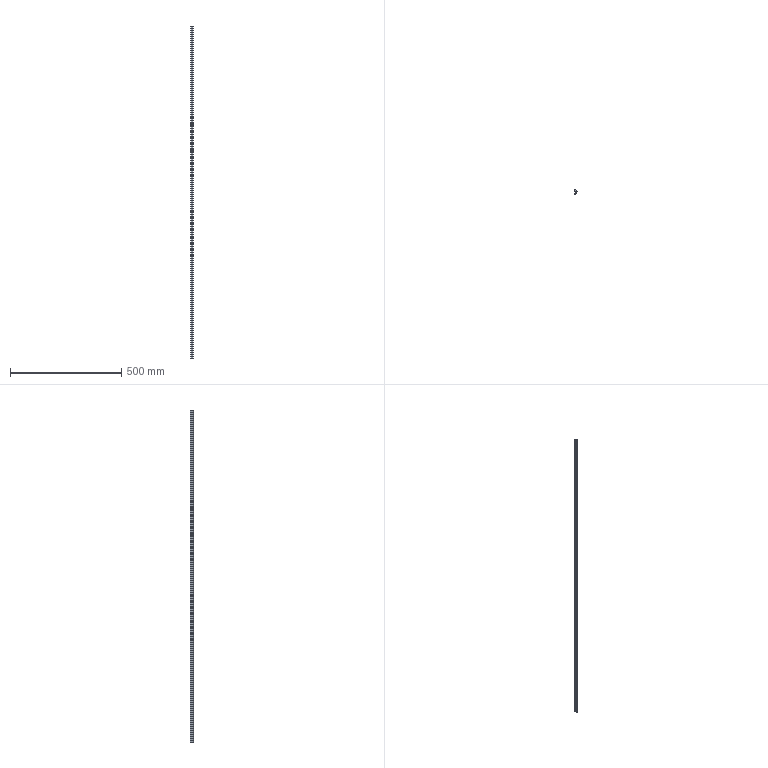Part | SolidWorks | features BaseBody 1, MoveFace 1 | 1 solid | 20 faces | box 10.8 x 17.5 x 1495 mm | volume 117807 mm3 | cylinder 11 | plane 9 | commonest cylinder face diameters 1.6 x2 14 x2 0.4 x1 0.6 x1 0.8 x1 2.6 x1
STEP:
#1=CARTESIAN_POINT('',(-3.236,-11.055,1395.));
#2=VERTEX_POINT('',#1);
#3=CARTESIAN_POINT('',(-4.3,-10.3,1395.));
#4=VERTEX_POINT('',#3);
#5=CARTESIAN_POINT('',(-3.5,-10.3,1395.));
#6=DIRECTION('',(0.,0.,-1.));
#7=DIRECTION('',(1.,0.,0.));
#8=AXIS2_PLACEMENT_3D('',#5,#6,#7);
#9=CIRCLE('',#8,0.8);
#10=EDGE_CURVE('',#2,#4,#9,.T.);
#11=ORIENTED_EDGE('',*,*,#10,.T.);
#12=CARTESIAN_POINT('',(-4.3,-10.3,-100.));
#13=VERTEX_POINT('',#12);
#14=CARTESIAN_POINT('',(-4.3,-10.3,-100.));
#15=DIRECTION('',(0.,0.,-1.));
#16=VECTOR('',#15,1000.);
#17=LINE('',#14,#16);
#18=EDGE_CURVE('',#4,#13,#17,.T.);
#19=ORIENTED_EDGE('',*,*,#18,.T.);
#20=CARTESIAN_POINT('',(-3.236,-11.055,-100.));
#21=VERTEX_POINT('',#20);
#22=CARTESIAN_POINT('',(-3.5,-10.3,-100.));
#23=DIRECTION('',(0.,0.,1.));
#24=DIRECTION('',(-1.,0.,0.));
#25=AXIS2_PLACEMENT_3D('',#22,#23,#24);
#26=CIRCLE('',#25,0.8);
#27=EDGE_CURVE('',#13,#21,#26,.T.);
#28=ORIENTED_EDGE('',*,*,#27,.T.);
#29=CARTESIAN_POINT('',(-3.236,-11.055,-100.));
#30=DIRECTION('',(0.,0.,-1.));
#31=VECTOR('',#30,1000.);
#32=LINE('',#29,#31);
#33=EDGE_CURVE('',#2,#21,#32,.T.);
#34=ORIENTED_EDGE('',*,*,#33,.F.);
#35=EDGE_LOOP('',(#11,#19,#28,#34));
#36=FACE_OUTER_BOUND('',#35,.T.);
#37=CARTESIAN_POINT('',(-3.5,-10.3,-100.));
#38=DIRECTION('',(0.,0.,-1.));
#39=DIRECTION('',(-1.,0.,0.));
#40=AXIS2_PLACEMENT_3D('',#37,#38,#39);
#41=CYLINDRICAL_SURFACE('',#40,0.8);
#42=ADVANCED_FACE('',(#36),#41,.T.);
#43=CARTESIAN_POINT('',(1.184,-6.397,-100.));
#44=VERTEX_POINT('',#43);
#45=CARTESIAN_POINT('',(-5.702,-4.29,-100.));
#46=DIRECTION('',(0.,0.,1.));
#47=DIRECTION('',(-1.,0.,0.));
#48=AXIS2_PLACEMENT_3D('',#45,#46,#47);
#49=CIRCLE('',#48,7.201);
#50=EDGE_CURVE('',#21,#44,#49,.T.);
#51=ORIENTED_EDGE('',*,*,#50,.T.);
#52=CARTESIAN_POINT('',(1.184,-6.397,1395.));
#53=VERTEX_POINT('',#52);
#54=CARTESIAN_POINT('',(1.184,-6.397,-100.));
#55=DIRECTION('',(0.,0.,1.));
#56=VECTOR('',#55,1000.);
#57=LINE('',#54,#56);
#58=EDGE_CURVE('',#44,#53,#57,.T.);
#59=ORIENTED_EDGE('',*,*,#58,.T.);
#60=CARTESIAN_POINT('',(-5.702,-4.29,1395.));
#61=DIRECTION('',(0.,0.,-1.));
#62=DIRECTION('',(1.,0.,0.));
#63=AXIS2_PLACEMENT_3D('',#60,#61,#62);
#64=CIRCLE('',#63,7.201);
#65=EDGE_CURVE('',#53,#2,#64,.T.);
#66=ORIENTED_EDGE('',*,*,#65,.T.);
#67=ORIENTED_EDGE('',*,*,#33,.T.);
#68=EDGE_LOOP('',(#51,#59,#66,#67));
#69=FACE_OUTER_BOUND('',#68,.T.);
#70=CARTESIAN_POINT('',(-5.702,-4.29,-100.));
#71=DIRECTION('',(0.,0.,-1.));
#72=DIRECTION('',(-1.,0.,0.));
#73=AXIS2_PLACEMENT_3D('',#70,#71,#72);
#74=CYLINDRICAL_SURFACE('',#73,7.201);
#75=ADVANCED_FACE('',(#69),#74,.T.);
#76=CARTESIAN_POINT('',(0.9,-6.,-100.));
#77=VERTEX_POINT('',#76);
#78=CARTESIAN_POINT('',(0.9,-6.3,-100.));
#79=DIRECTION('',(0.,0.,1.));
#80=DIRECTION('',(-1.,0.,0.));
#81=AXIS2_PLACEMENT_3D('',#78,#79,#80);
#82=CIRCLE('',#81,0.3);
#83=EDGE_CURVE('',#44,#77,#82,.T.);
#84=ORIENTED_EDGE('',*,*,#83,.T.);
#85=CARTESIAN_POINT('',(0.9,-6.,1395.));
#86=VERTEX_POINT('',#85);
#87=CARTESIAN_POINT('',(0.9,-6.,-100.));
#88=DIRECTION('',(0.,0.,1.));
#89=VECTOR('',#88,1000.);
#90=LINE('',#87,#89);
#91=EDGE_CURVE('',#77,#86,#90,.T.);
#92=ORIENTED_EDGE('',*,*,#91,.T.);
#93=CARTESIAN_POINT('',(0.9,-6.3,1395.));
#94=DIRECTION('',(0.,0.,-1.));
#95=DIRECTION('',(1.,0.,0.));
#96=AXIS2_PLACEMENT_3D('',#93,#94,#95);
#97=CIRCLE('',#96,0.3);
#98=EDGE_CURVE('',#86,#53,#97,.T.);
#99=ORIENTED_EDGE('',*,*,#98,.T.);
#100=ORIENTED_EDGE('',*,*,#58,.F.);
#101=EDGE_LOOP('',(#84,#92,#99,#100));
#102=FACE_OUTER_BOUND('',#101,.T.);
#103=CARTESIAN_POINT('',(0.9,-6.3,-100.));
#104=DIRECTION('',(0.,0.,-1.));
#105=DIRECTION('',(-1.,0.,0.));
#106=AXIS2_PLACEMENT_3D('',#103,#104,#105);
#107=CYLINDRICAL_SURFACE('',#106,0.3);
#108=ADVANCED_FACE('',(#102),#107,.T.);
#109=CARTESIAN_POINT('',(-2.5,-0.5,-100.));
#110=VERTEX_POINT('',#109);
#111=CARTESIAN_POINT('',(-2.5,-6.153,-100.));
#112=VERTEX_POINT('',#111);
#113=CARTESIAN_POINT('',(-2.5,-6.397,-100.));
#114=DIRECTION('',(0.,-1.,0.));
#115=VECTOR('',#114,1000.);
#116=LINE('',#113,#115);
#117=EDGE_CURVE('',#110,#112,#116,.T.);
#118=ORIENTED_EDGE('',*,*,#117,.F.);
#119=CARTESIAN_POINT('',(-4.2,1.695,-100.));
#120=VERTEX_POINT('',#119);
#121=CARTESIAN_POINT('',(-1.701,1.875,-100.));
#122=DIRECTION('',(0.,0.,1.));
#123=DIRECTION('',(-1.,0.,0.));
#124=AXIS2_PLACEMENT_3D('',#121,#122,#123);
#125=CIRCLE('',#124,2.506);
#126=EDGE_CURVE('',#120,#110,#125,.T.);
#127=ORIENTED_EDGE('',*,*,#126,.F.);
#128=CARTESIAN_POINT('',(-4.2,5.1,-100.));
#129=VERTEX_POINT('',#128);
#130=CARTESIAN_POINT('',(-4.2,-6.397,-100.));
#131=DIRECTION('',(0.,-1.,0.));
#132=VECTOR('',#131,1000.);
#133=LINE('',#130,#132);
#134=EDGE_CURVE('',#129,#120,#133,.T.);
#135=ORIENTED_EDGE('',*,*,#134,.F.);
#136=CARTESIAN_POINT('',(-2.892,6.4,-100.));
#137=VERTEX_POINT('',#136);
#138=CARTESIAN_POINT('',(-2.9,5.1,-100.));
#139=DIRECTION('',(0.,0.,1.));
#140=DIRECTION('',(-1.,0.,0.));
#141=AXIS2_PLACEMENT_3D('',#138,#139,#140);
#142=CIRCLE('',#141,1.3);
#143=EDGE_CURVE('',#137,#129,#142,.T.);
#144=ORIENTED_EDGE('',*,*,#143,.F.);
#145=CARTESIAN_POINT('',(0.5,5.5,-100.));
#146=VERTEX_POINT('',#145);
#147=CARTESIAN_POINT('',(-2.934,-0.5999,-100.));
#148=DIRECTION('',(0.,0.,1.));
#149=DIRECTION('',(-1.,0.,0.));
#150=AXIS2_PLACEMENT_3D('',#147,#148,#149);
#151=CIRCLE('',#150,7.);
#152=EDGE_CURVE('',#146,#137,#151,.T.);
#153=ORIENTED_EDGE('',*,*,#152,.F.);
#154=CARTESIAN_POINT('',(5.5,1.7,-100.));
#155=VERTEX_POINT('',#154);
#156=CARTESIAN_POINT('',(5.5,1.7,-100.));
#157=DIRECTION('',(-0.7962,0.6051,0.));
#158=VECTOR('',#157,1000.);
#159=LINE('',#156,#158);
#160=EDGE_CURVE('',#155,#146,#159,.T.);
#161=ORIENTED_EDGE('',*,*,#160,.F.);
#162=CARTESIAN_POINT('',(6.458,-0.2215,-100.));
#163=VERTEX_POINT('',#162);
#164=CARTESIAN_POINT('',(6.458,-0.2215,-100.));
#165=DIRECTION('',(-0.4462,0.8949,0.));
#166=VECTOR('',#165,1000.);
#167=LINE('',#164,#166);
#168=EDGE_CURVE('',#163,#155,#167,.T.);
#169=ORIENTED_EDGE('',*,*,#168,.F.);
#170=CARTESIAN_POINT('',(5.895,-0.7433,-100.));
#171=VERTEX_POINT('',#170);
#172=CARTESIAN_POINT('',(6.1,-0.4,-100.));
#173=DIRECTION('',(0.,0.,1.));
#174=DIRECTION('',(-1.,0.,0.));
#175=AXIS2_PLACEMENT_3D('',#172,#173,#174);
#176=CIRCLE('',#175,0.4);
#177=EDGE_CURVE('',#171,#163,#176,.T.);
#178=ORIENTED_EDGE('',*,*,#177,.F.);
#179=CARTESIAN_POINT('',(3.,0.,-100.));
#180=VERTEX_POINT('',#179);
#181=CARTESIAN_POINT('',(2.746,-6.995,-100.));
#182=DIRECTION('',(0.,0.,-1.));
#183=DIRECTION('',(-1.,0.,0.));
#184=AXIS2_PLACEMENT_3D('',#181,#182,#183);
#185=CIRCLE('',#184,7.);
#186=EDGE_CURVE('',#180,#171,#185,.T.);
#187=ORIENTED_EDGE('',*,*,#186,.F.);
#188=CARTESIAN_POINT('',(0.,0.,-100.));
#189=VERTEX_POINT('',#188);
#190=CARTESIAN_POINT('',(-6.814,0.,-100.));
#191=DIRECTION('',(1.,0.,0.));
#192=VECTOR('',#191,1000.);
#193=LINE('',#190,#192);
#194=EDGE_CURVE('',#189,#180,#193,.T.);
#195=ORIENTED_EDGE('',*,*,#194,.F.);
#196=CARTESIAN_POINT('',(0.,-5.8,-100.));
#197=VERTEX_POINT('',#196);
#198=CARTESIAN_POINT('',(0.,-6.397,-100.));
#199=DIRECTION('',(0.,1.,0.));
#200=VECTOR('',#199,1000.);
#201=LINE('',#198,#200);
#202=EDGE_CURVE('',#197,#189,#201,.T.);
#203=ORIENTED_EDGE('',*,*,#202,.F.);
#204=CARTESIAN_POINT('',(0.2,-6.,-100.));
#205=VERTEX_POINT('',#204);
#206=CARTESIAN_POINT('',(0.2,-5.8,-100.));
#207=DIRECTION('',(0.,0.,1.));
#208=DIRECTION('',(-1.,0.,0.));
#209=AXIS2_PLACEMENT_3D('',#206,#207,#208);
#210=CIRCLE('',#209,0.2);
#211=EDGE_CURVE('',#197,#205,#210,.T.);
#212=ORIENTED_EDGE('',*,*,#211,.T.);
#213=CARTESIAN_POINT('',(-6.814,-6.,-100.));
#214=DIRECTION('',(-1.,0.,0.));
#215=VECTOR('',#214,1000.);
#216=LINE('',#213,#215);
#217=EDGE_CURVE('',#77,#205,#216,.T.);
#218=ORIENTED_EDGE('',*,*,#217,.F.);
#219=ORIENTED_EDGE('',*,*,#83,.F.);
#220=ORIENTED_EDGE('',*,*,#50,.F.);
#221=ORIENTED_EDGE('',*,*,#27,.F.);
#222=CARTESIAN_POINT('',(-3.998,-9.674,-100.));
#223=VERTEX_POINT('',#222);
#224=CARTESIAN_POINT('',(-3.5,-10.3,-100.));
#225=DIRECTION('',(0.,0.,1.));
#226=DIRECTION('',(-1.,0.,0.));
#227=AXIS2_PLACEMENT_3D('',#224,#225,#226);
#228=CIRCLE('',#227,0.8);
#229=EDGE_CURVE('',#223,#13,#228,.T.);
#230=ORIENTED_EDGE('',*,*,#229,.F.);
#231=CARTESIAN_POINT('',(-6.814,-6.397,-100.));
#232=DIRECTION('',(0.,0.,-1.));
#233=DIRECTION('',(-1.,0.,0.));
#234=AXIS2_PLACEMENT_3D('',#231,#232,#233);
#235=CIRCLE('',#234,4.321);
#236=EDGE_CURVE('',#112,#223,#235,.T.);
#237=ORIENTED_EDGE('',*,*,#236,.F.);
#238=EDGE_LOOP('',(#118,#127,#135,#144,#153,#161,#169,#178,#187,#195,#203,#212,#218,#219,#220,#221,#230,#237));
#239=FACE_OUTER_BOUND('',#238,.T.);
#240=CARTESIAN_POINT('',(-6.814,-6.397,-100.));
#241=DIRECTION('',(0.,0.,1.));
#242=DIRECTION('',(1.,0.,0.));
#243=AXIS2_PLACEMENT_3D('',#240,#241,#242);
#244=PLANE('',#243);
#245=ADVANCED_FACE('',(#239),#244,.F.);
#246=ORIENTED_EDGE('',*,*,#18,.F.);
#247=CARTESIAN_POINT('',(-3.998,-9.674,1395.));
#248=VERTEX_POINT('',#247);
#249=CARTESIAN_POINT('',(-3.5,-10.3,1395.));
#250=DIRECTION('',(0.,0.,-1.));
#251=DIRECTION('',(1.,0.,0.));
#252=AXIS2_PLACEMENT_3D('',#249,#250,#251);
#253=CIRCLE('',#252,0.8);
#254=EDGE_CURVE('',#4,#248,#253,.T.);
#255=ORIENTED_EDGE('',*,*,#254,.T.);
#256=CARTESIAN_POINT('',(-3.998,-9.674,-100.));
#257=DIRECTION('',(0.,0.,-1.));
#258=VECTOR('',#257,1000.);
#259=LINE('',#256,#258);
#260=EDGE_CURVE('',#248,#223,#259,.T.);
#261=ORIENTED_EDGE('',*,*,#260,.T.);
#262=ORIENTED_EDGE('',*,*,#229,.T.);
#263=EDGE_LOOP('',(#246,#255,#261,#262));
#264=FACE_OUTER_BOUND('',#263,.T.);
#265=CARTESIAN_POINT('',(-3.5,-10.3,-100.));
#266=DIRECTION('',(0.,0.,-1.));
#267=DIRECTION('',(-1.,0.,0.));
#268=AXIS2_PLACEMENT_3D('',#265,#266,#267);
#269=CYLINDRICAL_SURFACE('',#268,0.8);
#270=ADVANCED_FACE('',(#264),#269,.T.);
#271=CARTESIAN_POINT('',(-4.2,1.695,1395.));
#272=VERTEX_POINT('',#271);
#273=CARTESIAN_POINT('',(-2.5,-0.5,1395.));
#274=VERTEX_POINT('',#273);
#275=CARTESIAN_POINT('',(-1.701,1.875,1395.));
#276=DIRECTION('',(0.,0.,1.));
#277=DIRECTION('',(1.,0.,0.));
#278=AXIS2_PLACEMENT_3D('',#275,#276,#277);
#279=CIRCLE('',#278,2.506);
#280=EDGE_CURVE('',#272,#274,#279,.T.);
#281=ORIENTED_EDGE('',*,*,#280,.T.);
#282=CARTESIAN_POINT('',(-2.5,-6.153,1395.));
#283=VERTEX_POINT('',#282);
#284=CARTESIAN_POINT('',(-2.5,-6.397,1395.));
#285=DIRECTION('',(0.,-1.,0.));
#286=VECTOR('',#285,1000.);
#287=LINE('',#284,#286);
#288=EDGE_CURVE('',#274,#283,#287,.T.);
#289=ORIENTED_EDGE('',*,*,#288,.T.);
#290=CARTESIAN_POINT('',(-6.814,-6.397,1395.));
#291=DIRECTION('',(0.,0.,-1.));
#292=DIRECTION('',(1.,0.,0.));
#293=AXIS2_PLACEMENT_3D('',#290,#291,#292);
#294=CIRCLE('',#293,4.321);
#295=EDGE_CURVE('',#283,#248,#294,.T.);
#296=ORIENTED_EDGE('',*,*,#295,.T.);
#297=ORIENTED_EDGE('',*,*,#254,.F.);
#298=ORIENTED_EDGE('',*,*,#10,.F.);
#299=ORIENTED_EDGE('',*,*,#65,.F.);
#300=ORIENTED_EDGE('',*,*,#98,.F.);
#301=CARTESIAN_POINT('',(0.2,-6.,1395.));
#302=VERTEX_POINT('',#301);
#303=CARTESIAN_POINT('',(-6.814,-6.,1395.));
#304=DIRECTION('',(-1.,0.,0.));
#305=VECTOR('',#304,1000.);
#306=LINE('',#303,#305);
#307=EDGE_CURVE('',#86,#302,#306,.T.);
#308=ORIENTED_EDGE('',*,*,#307,.T.);
#309=CARTESIAN_POINT('',(0.,-5.8,1395.));
#310=VERTEX_POINT('',#309);
#311=CARTESIAN_POINT('',(0.2,-5.8,1395.));
#312=DIRECTION('',(0.,0.,-1.));
#313=DIRECTION('',(1.,0.,0.));
#314=AXIS2_PLACEMENT_3D('',#311,#312,#313);
#315=CIRCLE('',#314,0.2);
#316=EDGE_CURVE('',#302,#310,#315,.T.);
#317=ORIENTED_EDGE('',*,*,#316,.T.);
#318=CARTESIAN_POINT('',(0.,0.,1395.));
#319=VERTEX_POINT('',#318);
#320=CARTESIAN_POINT('',(0.,-6.397,1395.));
#321=DIRECTION('',(0.,1.,0.));
#322=VECTOR('',#321,1000.);
#323=LINE('',#320,#322);
#324=EDGE_CURVE('',#310,#319,#323,.T.);
#325=ORIENTED_EDGE('',*,*,#324,.T.);
#326=CARTESIAN_POINT('',(3.,0.,1395.));
#327=VERTEX_POINT('',#326);
#328=CARTESIAN_POINT('',(-6.814,0.,1395.));
#329=DIRECTION('',(1.,0.,0.));
#330=VECTOR('',#329,1000.);
#331=LINE('',#328,#330);
#332=EDGE_CURVE('',#319,#327,#331,.T.);
#333=ORIENTED_EDGE('',*,*,#332,.T.);
#334=CARTESIAN_POINT('',(5.895,-0.7433,1395.));
#335=VERTEX_POINT('',#334);
#336=CARTESIAN_POINT('',(2.746,-6.995,1395.));
#337=DIRECTION('',(0.,0.,-1.));
#338=DIRECTION('',(1.,0.,0.));
#339=AXIS2_PLACEMENT_3D('',#336,#337,#338);
#340=CIRCLE('',#339,7.);
#341=EDGE_CURVE('',#327,#335,#340,.T.);
#342=ORIENTED_EDGE('',*,*,#341,.T.);
#343=CARTESIAN_POINT('',(6.458,-0.2215,1395.));
#344=VERTEX_POINT('',#343);
#345=CARTESIAN_POINT('',(6.1,-0.4,1395.));
#346=DIRECTION('',(0.,0.,-1.));
#347=DIRECTION('',(1.,0.,0.));
#348=AXIS2_PLACEMENT_3D('',#345,#346,#347);
#349=CIRCLE('',#348,0.4);
#350=EDGE_CURVE('',#344,#335,#349,.T.);
#351=ORIENTED_EDGE('',*,*,#350,.F.);
#352=CARTESIAN_POINT('',(5.5,1.7,1395.));
#353=VERTEX_POINT('',#352);
#354=CARTESIAN_POINT('',(6.282,0.1323,1395.));
#355=DIRECTION('',(-0.4462,0.8949,0.));
#356=VECTOR('',#355,1000.);
#357=LINE('',#354,#356);
#358=EDGE_CURVE('',#344,#353,#357,.T.);
#359=ORIENTED_EDGE('',*,*,#358,.T.);
#360=CARTESIAN_POINT('',(0.5,5.5,1395.));
#361=VERTEX_POINT('',#360);
#362=CARTESIAN_POINT('',(1.595,4.668,1395.));
#363=DIRECTION('',(-0.7962,0.6051,0.));
#364=VECTOR('',#363,1000.);
#365=LINE('',#362,#364);
#366=EDGE_CURVE('',#353,#361,#365,.T.);
#367=ORIENTED_EDGE('',*,*,#366,.T.);
#368=CARTESIAN_POINT('',(-2.892,6.4,1395.));
#369=VERTEX_POINT('',#368);
#370=CARTESIAN_POINT('',(-2.934,-0.5999,1395.));
#371=DIRECTION('',(0.,0.,1.));
#372=DIRECTION('',(1.,0.,0.));
#373=AXIS2_PLACEMENT_3D('',#370,#371,#372);
#374=CIRCLE('',#373,7.);
#375=EDGE_CURVE('',#361,#369,#374,.T.);
#376=ORIENTED_EDGE('',*,*,#375,.T.);
#377=CARTESIAN_POINT('',(-4.2,5.1,1395.));
#378=VERTEX_POINT('',#377);
#379=CARTESIAN_POINT('',(-2.9,5.1,1395.));
#380=DIRECTION('',(0.,0.,1.));
#381=DIRECTION('',(1.,0.,0.));
#382=AXIS2_PLACEMENT_3D('',#379,#380,#381);
#383=CIRCLE('',#382,1.3);
#384=EDGE_CURVE('',#369,#378,#383,.T.);
#385=ORIENTED_EDGE('',*,*,#384,.T.);
#386=CARTESIAN_POINT('',(-4.2,-6.397,1395.));
#387=DIRECTION('',(0.,-1.,0.));
#388=VECTOR('',#387,1000.);
#389=LINE('',#386,#388);
#390=EDGE_CURVE('',#378,#272,#389,.T.);
#391=ORIENTED_EDGE('',*,*,#390,.T.);
#392=EDGE_LOOP('',(#281,#289,#296,#297,#298,#299,#300,#308,#317,#325,#333,#342,#351,#359,#367,#376,#385,#391));
#393=FACE_OUTER_BOUND('',#392,.T.);
#394=CARTESIAN_POINT('',(-6.814,-6.397,1395.));
#395=DIRECTION('',(0.,0.,1.));
#396=DIRECTION('',(1.,0.,0.));
#397=AXIS2_PLACEMENT_3D('',#394,#395,#396);
#398=PLANE('',#397);
#399=ADVANCED_FACE('',(#393),#398,.T.);
#400=ORIENTED_EDGE('',*,*,#217,.T.);
#401=CARTESIAN_POINT('',(0.2,-6.,-100.));
#402=DIRECTION('',(0.,0.,1.));
#403=VECTOR('',#402,1000.);
#404=LINE('',#401,#403);
#405=EDGE_CURVE('',#205,#302,#404,.T.);
#406=ORIENTED_EDGE('',*,*,#405,.T.);
#407=ORIENTED_EDGE('',*,*,#307,.F.);
#408=ORIENTED_EDGE('',*,*,#91,.F.);
#409=EDGE_LOOP('',(#400,#406,#407,#408));
#410=FACE_OUTER_BOUND('',#409,.T.);
#411=CARTESIAN_POINT('',(0.9,-6.,-100.));
#412=DIRECTION('',(0.,1.,0.));
#413=DIRECTION('',(0.,0.,1.));
#414=AXIS2_PLACEMENT_3D('',#411,#412,#413);
#415=PLANE('',#414);
#416=ADVANCED_FACE('',(#410),#415,.T.);
#417=CARTESIAN_POINT('',(-2.5,-6.153,-100.));
#418=DIRECTION('',(0.,0.,1.));
#419=VECTOR('',#418,1000.);
#420=LINE('',#417,#419);
#421=EDGE_CURVE('',#112,#283,#420,.T.);
#422=ORIENTED_EDGE('',*,*,#421,.F.);
#423=ORIENTED_EDGE('',*,*,#236,.T.);
#424=ORIENTED_EDGE('',*,*,#260,.F.);
#425=ORIENTED_EDGE('',*,*,#295,.F.);
#426=EDGE_LOOP('',(#422,#423,#424,#425));
#427=FACE_OUTER_BOUND('',#426,.T.);
#428=CARTESIAN_POINT('',(-6.814,-6.397,-100.));
#429=DIRECTION('',(0.,0.,-1.));
#430=DIRECTION('',(-1.,0.,0.));
#431=AXIS2_PLACEMENT_3D('',#428,#429,#430);
#432=CYLINDRICAL_SURFACE('',#431,4.321);
#433=ADVANCED_FACE('',(#427),#432,.F.);
#434=ORIENTED_EDGE('',*,*,#117,.T.);
#435=ORIENTED_EDGE('',*,*,#421,.T.);
#436=ORIENTED_EDGE('',*,*,#288,.F.);
#437=CARTESIAN_POINT('',(-2.5,-0.5,-100.));
#438=DIRECTION('',(0.,0.,-1.));
#439=VECTOR('',#438,1000.);
#440=LINE('',#437,#439);
#441=EDGE_CURVE('',#274,#110,#440,.T.);
#442=ORIENTED_EDGE('',*,*,#441,.T.);
#443=EDGE_LOOP('',(#434,#435,#436,#442));
#444=FACE_OUTER_BOUND('',#443,.T.);
#445=CARTESIAN_POINT('',(-2.5,-0.5,-100.));
#446=DIRECTION('',(-1.,0.,0.));
#447=DIRECTION('',(0.,0.,1.));
#448=AXIS2_PLACEMENT_3D('',#445,#446,#447);
#449=PLANE('',#448);
#450=ADVANCED_FACE('',(#444),#449,.T.);
#451=ORIENTED_EDGE('',*,*,#126,.T.);
#452=ORIENTED_EDGE('',*,*,#441,.F.);
#453=ORIENTED_EDGE('',*,*,#280,.F.);
#454=CARTESIAN_POINT('',(-4.2,1.695,-100.));
#455=DIRECTION('',(0.,0.,-1.));
#456=VECTOR('',#455,1000.);
#457=LINE('',#454,#456);
#458=EDGE_CURVE('',#272,#120,#457,.T.);
#459=ORIENTED_EDGE('',*,*,#458,.T.);
#460=EDGE_LOOP('',(#451,#452,#453,#459));
#461=FACE_OUTER_BOUND('',#460,.T.);
#462=CARTESIAN_POINT('',(-1.701,1.875,-100.));
#463=DIRECTION('',(0.,0.,-1.));
#464=DIRECTION('',(-1.,0.,0.));
#465=AXIS2_PLACEMENT_3D('',#462,#463,#464);
#466=CYLINDRICAL_SURFACE('',#465,2.506);
#467=ADVANCED_FACE('',(#461),#466,.T.);
#468=ORIENTED_EDGE('',*,*,#134,.T.);
#469=ORIENTED_EDGE('',*,*,#458,.F.);
#470=ORIENTED_EDGE('',*,*,#390,.F.);
#471=CARTESIAN_POINT('',(-4.2,5.1,-100.));
#472=DIRECTION('',(0.,0.,-1.));
#473=VECTOR('',#472,1000.);
#474=LINE('',#471,#473);
#475=EDGE_CURVE('',#378,#129,#474,.T.);
#476=ORIENTED_EDGE('',*,*,#475,.T.);
#477=EDGE_LOOP('',(#468,#469,#470,#476));
#478=FACE_OUTER_BOUND('',#477,.T.);
#479=CARTESIAN_POINT('',(-4.2,5.1,-100.));
#480=DIRECTION('',(-1.,0.,0.));
#481=DIRECTION('',(0.,0.,1.));
#482=AXIS2_PLACEMENT_3D('',#479,#480,#481);
#483=PLANE('',#482);
#484=ADVANCED_FACE('',(#478),#483,.T.);
#485=ORIENTED_EDGE('',*,*,#143,.T.);
#486=ORIENTED_EDGE('',*,*,#475,.F.);
#487=ORIENTED_EDGE('',*,*,#384,.F.);
#488=CARTESIAN_POINT('',(-2.892,6.4,-100.));
#489=DIRECTION('',(0.,0.,-1.));
#490=VECTOR('',#489,1000.);
#491=LINE('',#488,#490);
#492=EDGE_CURVE('',#369,#137,#491,.T.);
#493=ORIENTED_EDGE('',*,*,#492,.T.);
#494=EDGE_LOOP('',(#485,#486,#487,#493));
#495=FACE_OUTER_BOUND('',#494,.T.);
#496=CARTESIAN_POINT('',(-2.9,5.1,-100.));
#497=DIRECTION('',(0.,0.,-1.));
#498=DIRECTION('',(-1.,0.,0.));
#499=AXIS2_PLACEMENT_3D('',#496,#497,#498);
#500=CYLINDRICAL_SURFACE('',#499,1.3);
#501=ADVANCED_FACE('',(#495),#500,.T.);
#502=ORIENTED_EDGE('',*,*,#152,.T.);
#503=ORIENTED_EDGE('',*,*,#492,.F.);
#504=ORIENTED_EDGE('',*,*,#375,.F.);
#505=CARTESIAN_POINT('',(0.5,5.5,-100.));
#506=DIRECTION('',(0.,0.,-1.));
#507=VECTOR('',#506,1000.);
#508=LINE('',#505,#507);
#509=EDGE_CURVE('',#361,#146,#508,.T.);
#510=ORIENTED_EDGE('',*,*,#509,.T.);
#511=EDGE_LOOP('',(#502,#503,#504,#510));
#512=FACE_OUTER_BOUND('',#511,.T.);
#513=CARTESIAN_POINT('',(-2.934,-0.5999,-100.));
#514=DIRECTION('',(0.,0.,-1.));
#515=DIRECTION('',(-1.,0.,0.));
#516=AXIS2_PLACEMENT_3D('',#513,#514,#515);
#517=CYLINDRICAL_SURFACE('',#516,7.);
#518=ADVANCED_FACE('',(#512),#517,.T.);
#519=ORIENTED_EDGE('',*,*,#160,.T.);
#520=ORIENTED_EDGE('',*,*,#509,.F.);
#521=ORIENTED_EDGE('',*,*,#366,.F.);
#522=CARTESIAN_POINT('',(5.5,1.7,-100.));
#523=DIRECTION('',(0.,0.,-1.));
#524=VECTOR('',#523,1000.);
#525=LINE('',#522,#524);
#526=EDGE_CURVE('',#353,#155,#525,.T.);
#527=ORIENTED_EDGE('',*,*,#526,.T.);
#528=EDGE_LOOP('',(#519,#520,#521,#527));
#529=FACE_OUTER_BOUND('',#528,.T.);
#530=CARTESIAN_POINT('',(5.5,1.7,-100.));
#531=DIRECTION('',(0.6051,0.7962,0.));
#532=DIRECTION('',(-0.7962,0.6051,0.));
#533=AXIS2_PLACEMENT_3D('',#530,#531,#532);
#534=PLANE('',#533);
#535=ADVANCED_FACE('',(#529),#534,.T.);
#536=ORIENTED_EDGE('',*,*,#168,.T.);
#537=ORIENTED_EDGE('',*,*,#526,.F.);
#538=ORIENTED_EDGE('',*,*,#358,.F.);
#539=CARTESIAN_POINT('',(6.458,-0.2215,-100.));
#540=DIRECTION('',(0.,0.,-1.));
#541=VECTOR('',#540,1000.);
#542=LINE('',#539,#541);
#543=EDGE_CURVE('',#344,#163,#542,.T.);
#544=ORIENTED_EDGE('',*,*,#543,.T.);
#545=EDGE_LOOP('',(#536,#537,#538,#544));
#546=FACE_OUTER_BOUND('',#545,.T.);
#547=CARTESIAN_POINT('',(6.458,-0.2215,-100.));
#548=DIRECTION('',(0.8949,0.4462,0.));
#549=DIRECTION('',(-0.4462,0.8949,0.));
#550=AXIS2_PLACEMENT_3D('',#547,#548,#549);
#551=PLANE('',#550);
#552=ADVANCED_FACE('',(#546),#551,.T.);
#553=CARTESIAN_POINT('',(3.,0.,-100.));
#554=DIRECTION('',(0.,0.,1.));
#555=VECTOR('',#554,1000.);
#556=LINE('',#553,#555);
#557=EDGE_CURVE('',#180,#327,#556,.T.);
#558=ORIENTED_EDGE('',*,*,#557,.F.);
#559=ORIENTED_EDGE('',*,*,#186,.T.);
#560=CARTESIAN_POINT('',(5.895,-0.7433,-100.));
#561=DIRECTION('',(0.,0.,-1.));
#562=VECTOR('',#561,1000.);
#563=LINE('',#560,#562);
#564=EDGE_CURVE('',#335,#171,#563,.T.);
#565=ORIENTED_EDGE('',*,*,#564,.F.);
#566=ORIENTED_EDGE('',*,*,#341,.F.);
#567=EDGE_LOOP('',(#558,#559,#565,#566));
#568=FACE_OUTER_BOUND('',#567,.T.);
#569=CARTESIAN_POINT('',(2.746,-6.995,-100.));
#570=DIRECTION('',(0.,0.,-1.));
#571=DIRECTION('',(-1.,0.,0.));
#572=AXIS2_PLACEMENT_3D('',#569,#570,#571);
#573=CYLINDRICAL_SURFACE('',#572,7.);
#574=ADVANCED_FACE('',(#568),#573,.F.);
#575=ORIENTED_EDGE('',*,*,#194,.T.);
#576=ORIENTED_EDGE('',*,*,#557,.T.);
#577=ORIENTED_EDGE('',*,*,#332,.F.);
#578=CARTESIAN_POINT('',(0.,0.,-100.));
#579=DIRECTION('',(0.,0.,-1.));
#580=VECTOR('',#579,1000.);
#581=LINE('',#578,#580);
#582=EDGE_CURVE('',#319,#189,#581,.T.);
#583=ORIENTED_EDGE('',*,*,#582,.T.);
#584=EDGE_LOOP('',(#575,#576,#577,#583));
#585=FACE_OUTER_BOUND('',#584,.T.);
#586=CARTESIAN_POINT('',(0.,0.,-100.));
#587=DIRECTION('',(0.,-1.,0.));
#588=DIRECTION('',(0.,0.,-1.));
#589=AXIS2_PLACEMENT_3D('',#586,#587,#588);
#590=PLANE('',#589);
#591=ADVANCED_FACE('',(#585),#590,.T.);
#592=ORIENTED_EDGE('',*,*,#202,.T.);
#593=ORIENTED_EDGE('',*,*,#582,.F.);
#594=ORIENTED_EDGE('',*,*,#324,.F.);
#595=CARTESIAN_POINT('',(0.,-5.8,-100.));
#596=DIRECTION('',(0.,0.,-1.));
#597=VECTOR('',#596,1000.);
#598=LINE('',#595,#597);
#599=EDGE_CURVE('',#310,#197,#598,.T.);
#600=ORIENTED_EDGE('',*,*,#599,.T.);
#601=EDGE_LOOP('',(#592,#593,#594,#600));
#602=FACE_OUTER_BOUND('',#601,.T.);
#603=CARTESIAN_POINT('',(0.,-5.8,-100.));
#604=DIRECTION('',(1.,0.,0.));
#605=DIRECTION('',(0.,0.,-1.));
#606=AXIS2_PLACEMENT_3D('',#603,#604,#605);
#607=PLANE('',#606);
#608=ADVANCED_FACE('',(#602),#607,.T.);
#609=ORIENTED_EDGE('',*,*,#405,.F.);
#610=ORIENTED_EDGE('',*,*,#211,.F.);
#611=ORIENTED_EDGE('',*,*,#599,.F.);
#612=ORIENTED_EDGE('',*,*,#316,.F.);
#613=EDGE_LOOP('',(#609,#610,#611,#612));
#614=FACE_OUTER_BOUND('',#613,.T.);
#615=CARTESIAN_POINT('',(0.2,-5.8,-100.));
#616=DIRECTION('',(0.,0.,-1.));
#617=DIRECTION('',(-1.,0.,0.));
#618=AXIS2_PLACEMENT_3D('',#615,#616,#617);
#619=CYLINDRICAL_SURFACE('',#618,0.2);
#620=ADVANCED_FACE('',(#614),#619,.F.);
#621=ORIENTED_EDGE('',*,*,#177,.T.);
#622=ORIENTED_EDGE('',*,*,#543,.F.);
#623=ORIENTED_EDGE('',*,*,#350,.T.);
#624=ORIENTED_EDGE('',*,*,#564,.T.);
#625=EDGE_LOOP('',(#621,#622,#623,#624));
#626=FACE_OUTER_BOUND('',#625,.T.);
#627=CARTESIAN_POINT('',(6.1,-0.4,-100.));
#628=DIRECTION('',(0.,0.,-1.));
#629=DIRECTION('',(-1.,0.,0.));
#630=AXIS2_PLACEMENT_3D('',#627,#628,#629);
#631=CYLINDRICAL_SURFACE('',#630,0.4);
#632=ADVANCED_FACE('',(#626),#631,.T.);
#633=CLOSED_SHELL('',(#42,#75,#108,#245,#270,#399,#416,#433,#450,#467,#484,#501,#518,#535,#552,#574,#591,#608,#620,#632));
#634=MANIFOLD_SOLID_BREP('',#633);
#635=CARTESIAN_POINT('',(0.,0.,0.));
#636=DIRECTION('',(0.,0.,1.));
#637=DIRECTION('',(1.,0.,0.));
#638=AXIS2_PLACEMENT_3D('',#635,#636,#637);
#639=(LENGTH_UNIT()NAMED_UNIT(*)SI_UNIT(.MILLI.,.METRE.));
#640=UNCERTAINTY_MEASURE_WITH_UNIT(LENGTH_MEASURE(0.00001),#639,'','');
#641=(NAMED_UNIT(*)PLANE_ANGLE_UNIT()SI_UNIT($,.RADIAN.));
#642=(NAMED_UNIT(*)SI_UNIT($,.STERADIAN.)SOLID_ANGLE_UNIT());
#643=(GEOMETRIC_REPRESENTATION_CONTEXT(3)GLOBAL_UNCERTAINTY_ASSIGNED_CONTEXT((#640))GLOBAL_UNIT_ASSIGNED_CONTEXT((#639,#641,#642))REPRESENTATION_CONTEXT('',''));
#644=ADVANCED_BREP_SHAPE_REPRESENTATION('',(#634,#638),#643);